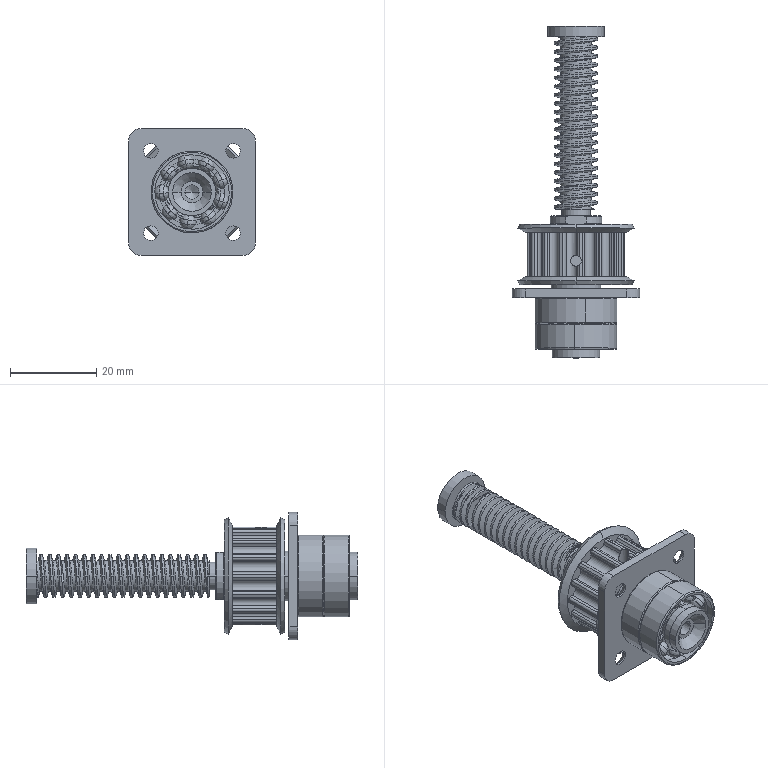Part | NX | features BREP 9 | 12 solids | 546 faces | box 29.5 x 77 x 29.5 mm | volume 11213 mm3 | cylinder 245 | sphere 144 | plane 82 | cone 45 | torus 28 | spline 2 | commonest cylinder face diameters 1.02 x42 10 x41 5.08 x33 2.74 x21 22.73 x15 17.3 x12